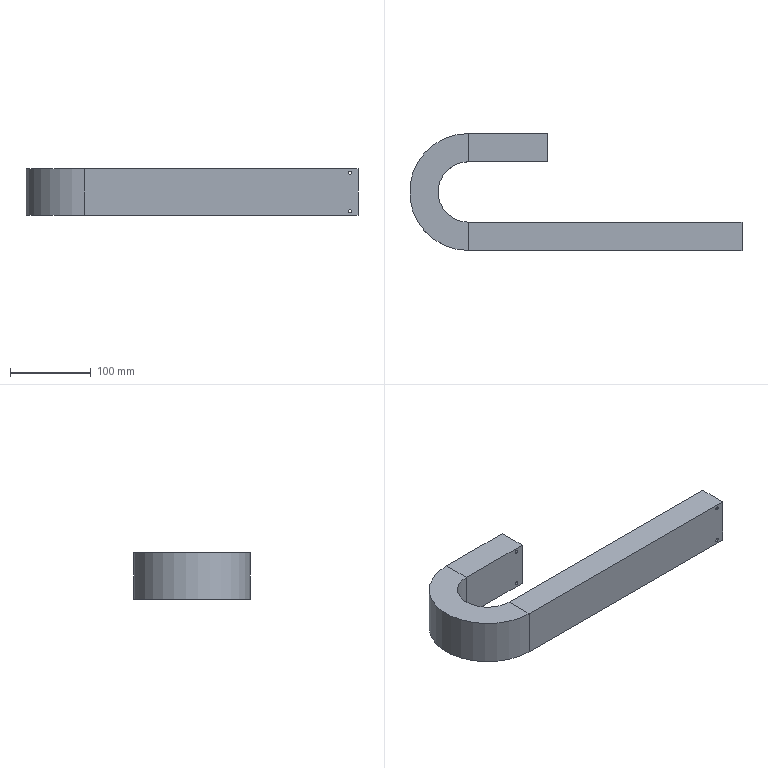Part | STEP file | Quiet two-side-openable cable carrier JFLO25x38-R55-25 links | 1 solid | 34 faces | box 412 x 145 x 58 mm | volume 657351 mm3 | plane 22 | cylinder 12 | commonest cylinder face diameters 4 x8 75 x1 85 x1 135 x1 145 x1